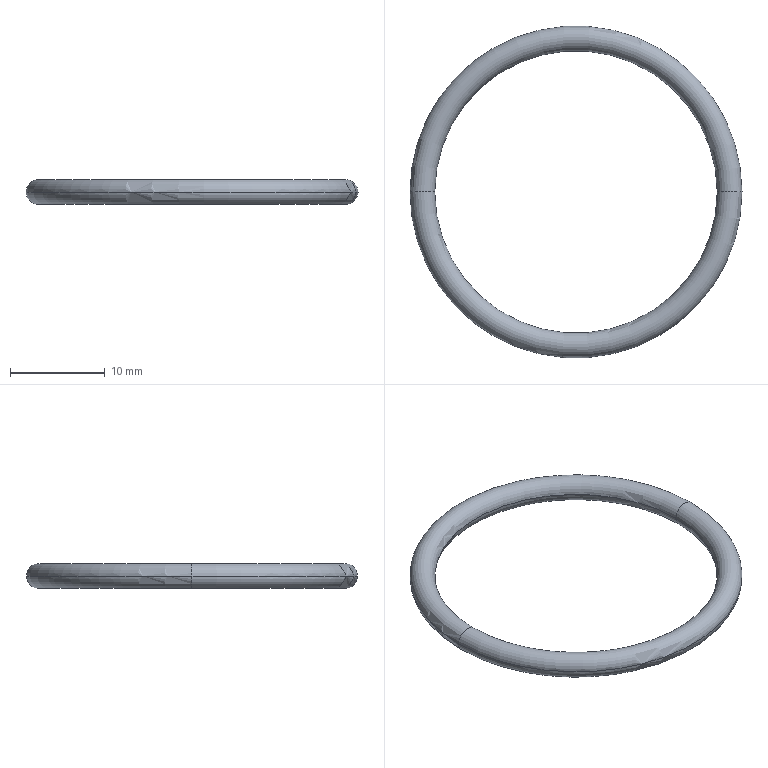Part | NX | features REVOLVE1 2 | 1 solid | 4 faces | box 35.052 x 35.052 x 2.616 mm | volume 547.78 mm3 | torus 4
STEP:
#1=CARTESIAN_POINT('',(-17.526,0.,0.));
#2=VERTEX_POINT('',#1);
#3=CARTESIAN_POINT('',(-14.91,0.,0.));
#4=VERTEX_POINT('',#3);
#5=CARTESIAN_POINT('',(-16.218,0.,0.));
#6=DIRECTION('',(0.,1.,0.));
#7=DIRECTION('',(-1.,0.,0.));
#8=AXIS2_PLACEMENT_3D('',#5,#6,#7);
#9=CIRCLE('',#8,1.308);
#10=EDGE_CURVE('',#2,#4,#9,.T.);
#11=ORIENTED_EDGE('',*,*,#10,.F.);
#12=CARTESIAN_POINT('',(17.526,0.,0.));
#13=VERTEX_POINT('',#12);
#14=CARTESIAN_POINT('',(0.,0.,0.));
#15=DIRECTION('',(0.,0.,1.));
#16=DIRECTION('',(1.,0.,0.));
#17=AXIS2_PLACEMENT_3D('',#14,#15,#16);
#18=CIRCLE('',#17,17.526);
#19=EDGE_CURVE('',#2,#13,#18,.T.);
#20=ORIENTED_EDGE('',*,*,#19,.T.);
#21=CARTESIAN_POINT('',(14.91,0.,0.));
#22=VERTEX_POINT('',#21);
#23=CARTESIAN_POINT('',(16.218,0.,0.));
#24=DIRECTION('',(0.,-1.,0.));
#25=DIRECTION('',(0.,0.,-1.));
#26=AXIS2_PLACEMENT_3D('',#23,#24,#25);
#27=CIRCLE('',#26,1.308);
#28=EDGE_CURVE('',#22,#13,#27,.F.);
#29=ORIENTED_EDGE('',*,*,#28,.F.);
#30=CARTESIAN_POINT('',(0.,0.,0.));
#31=DIRECTION('',(0.,0.,1.));
#32=DIRECTION('',(1.,0.,0.));
#33=AXIS2_PLACEMENT_3D('',#30,#31,#32);
#34=CIRCLE('',#33,14.91);
#35=EDGE_CURVE('',#22,#4,#34,.F.);
#36=ORIENTED_EDGE('',*,*,#35,.T.);
#37=EDGE_LOOP('',(#11,#20,#29,#36));
#38=FACE_BOUND('',#37,.T.);
#39=CARTESIAN_POINT('',(0.,0.,0.));
#40=DIRECTION('',(0.,0.,1.));
#41=DIRECTION('',(-1.,0.,0.));
#42=AXIS2_PLACEMENT_3D('',#39,#40,#41);
#43=TOROIDAL_SURFACE('',#42,16.218,1.308);
#44=ADVANCED_FACE('',(#38),#43,.T.);
#45=ORIENTED_EDGE('',*,*,#28,.T.);
#46=CARTESIAN_POINT('',(0.,0.,0.));
#47=DIRECTION('',(0.,0.,1.));
#48=DIRECTION('',(1.,0.,0.));
#49=AXIS2_PLACEMENT_3D('',#46,#47,#48);
#50=CIRCLE('',#49,17.526);
#51=EDGE_CURVE('',#13,#2,#50,.T.);
#52=ORIENTED_EDGE('',*,*,#51,.T.);
#53=ORIENTED_EDGE('',*,*,#10,.T.);
#54=CARTESIAN_POINT('',(0.,0.,0.));
#55=DIRECTION('',(0.,0.,1.));
#56=DIRECTION('',(1.,0.,0.));
#57=AXIS2_PLACEMENT_3D('',#54,#55,#56);
#58=CIRCLE('',#57,14.91);
#59=EDGE_CURVE('',#4,#22,#58,.F.);
#60=ORIENTED_EDGE('',*,*,#59,.T.);
#61=EDGE_LOOP('',(#45,#52,#53,#60));
#62=FACE_BOUND('',#61,.T.);
#63=CARTESIAN_POINT('',(0.,0.,0.));
#64=DIRECTION('',(0.,0.,1.));
#65=DIRECTION('',(-1.,0.,0.));
#66=AXIS2_PLACEMENT_3D('',#63,#64,#65);
#67=TOROIDAL_SURFACE('',#66,16.218,1.308);
#68=ADVANCED_FACE('',(#62),#67,.T.);
#69=ORIENTED_EDGE('',*,*,#51,.F.);
#70=CARTESIAN_POINT('',(16.218,0.,0.));
#71=DIRECTION('',(0.,-1.,0.));
#72=DIRECTION('',(0.,0.,-1.));
#73=AXIS2_PLACEMENT_3D('',#70,#71,#72);
#74=CIRCLE('',#73,1.308);
#75=EDGE_CURVE('',#13,#22,#74,.F.);
#76=ORIENTED_EDGE('',*,*,#75,.T.);
#77=ORIENTED_EDGE('',*,*,#59,.F.);
#78=CARTESIAN_POINT('',(-16.218,0.,0.));
#79=DIRECTION('',(0.,1.,0.));
#80=DIRECTION('',(-1.,0.,0.));
#81=AXIS2_PLACEMENT_3D('',#78,#79,#80);
#82=CIRCLE('',#81,1.308);
#83=EDGE_CURVE('',#4,#2,#82,.T.);
#84=ORIENTED_EDGE('',*,*,#83,.T.);
#85=EDGE_LOOP('',(#69,#76,#77,#84));
#86=FACE_BOUND('',#85,.T.);
#87=CARTESIAN_POINT('',(0.,0.,0.));
#88=DIRECTION('',(0.,0.,1.));
#89=DIRECTION('',(-1.,0.,0.));
#90=AXIS2_PLACEMENT_3D('',#87,#88,#89);
#91=TOROIDAL_SURFACE('',#90,16.218,1.308);
#92=ADVANCED_FACE('',(#86),#91,.T.);
#93=ORIENTED_EDGE('',*,*,#19,.F.);
#94=ORIENTED_EDGE('',*,*,#83,.F.);
#95=ORIENTED_EDGE('',*,*,#35,.F.);
#96=ORIENTED_EDGE('',*,*,#75,.F.);
#97=EDGE_LOOP('',(#93,#94,#95,#96));
#98=FACE_BOUND('',#97,.T.);
#99=CARTESIAN_POINT('',(0.,0.,0.));
#100=DIRECTION('',(0.,0.,1.));
#101=DIRECTION('',(-1.,0.,0.));
#102=AXIS2_PLACEMENT_3D('',#99,#100,#101);
#103=TOROIDAL_SURFACE('',#102,16.218,1.308);
#104=ADVANCED_FACE('',(#98),#103,.T.);
#105=CLOSED_SHELL('',(#44,#68,#92,#104));
#106=MANIFOLD_SOLID_BREP('',#105);
#107=(LENGTH_UNIT()NAMED_UNIT(*)SI_UNIT(.MILLI.,.METRE.));
#108=UNCERTAINTY_MEASURE_WITH_UNIT(LENGTH_MEASURE(0.00001),#107,'','');
#109=(NAMED_UNIT(*)PLANE_ANGLE_UNIT()SI_UNIT($,.RADIAN.));
#110=(NAMED_UNIT(*)SI_UNIT($,.STERADIAN.)SOLID_ANGLE_UNIT());
#111=(GEOMETRIC_REPRESENTATION_CONTEXT(3)GLOBAL_UNCERTAINTY_ASSIGNED_CONTEXT((#108))GLOBAL_UNIT_ASSIGNED_CONTEXT((#107,#109,#110))REPRESENTATION_CONTEXT('',''));
#112=ADVANCED_BREP_SHAPE_REPRESENTATION('',(#106),#111);